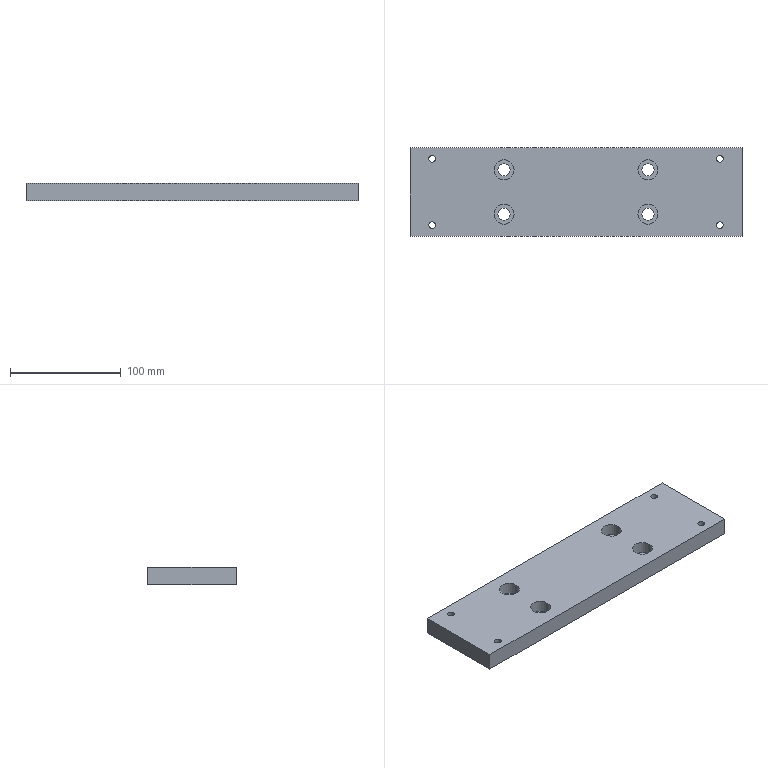Part | STEP file | PN_0009 connecting plate2 | 1 solid | 34 faces | box 300 x 80 x 16 mm | volume 369093 mm3 | cylinder 24 | plane 10 | commonest cylinder face diameters 6 x8 11 x8 18 x8